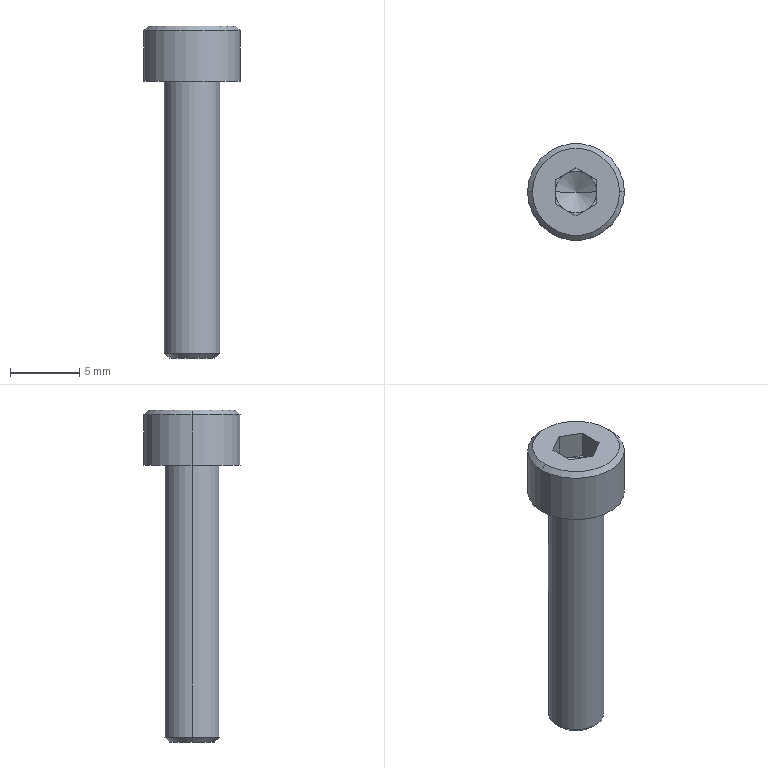Part | SolidWorks | features BaseBody 1 | 1 solid | 25 faces | box 7 x 7 x 24 mm | volume 385.61 mm3 | plane 15 | cone 6 | cylinder 4 | commonest cylinder face diameters 4 x2 7 x2
STEP:
#1=CARTESIAN_POINT('',(2.,0.,-19.65));
#2=VERTEX_POINT('',#1);
#3=CARTESIAN_POINT('',(-2.,0.,-19.65));
#4=VERTEX_POINT('',#3);
#5=CARTESIAN_POINT('',(0.,0.,-19.65));
#6=DIRECTION('',(0.,0.,1.));
#7=DIRECTION('',(1.,0.,0.));
#8=AXIS2_PLACEMENT_3D('',#5,#6,#7);
#9=CIRCLE('',#8,2.);
#10=EDGE_CURVE('',#2,#4,#9,.T.);
#11=ORIENTED_EDGE('',*,*,#10,.T.);
#12=CARTESIAN_POINT('',(-2.,0.,0.));
#13=VERTEX_POINT('',#12);
#14=CARTESIAN_POINT('',(-2.,0.,-20.));
#15=DIRECTION('',(0.,0.,1.));
#16=VECTOR('',#15,1000.);
#17=LINE('',#14,#16);
#18=EDGE_CURVE('',#4,#13,#17,.T.);
#19=ORIENTED_EDGE('',*,*,#18,.T.);
#20=CARTESIAN_POINT('',(2.,0.,0.));
#21=VERTEX_POINT('',#20);
#22=CARTESIAN_POINT('',(0.,0.,0.));
#23=DIRECTION('',(0.,0.,-1.));
#24=DIRECTION('',(1.,0.,0.));
#25=AXIS2_PLACEMENT_3D('',#22,#23,#24);
#26=CIRCLE('',#25,2.);
#27=EDGE_CURVE('',#13,#21,#26,.T.);
#28=ORIENTED_EDGE('',*,*,#27,.T.);
#29=CARTESIAN_POINT('',(2.,0.,-20.));
#30=DIRECTION('',(0.,0.,1.));
#31=VECTOR('',#30,1000.);
#32=LINE('',#29,#31);
#33=EDGE_CURVE('',#2,#21,#32,.T.);
#34=ORIENTED_EDGE('',*,*,#33,.F.);
#35=EDGE_LOOP('',(#11,#19,#28,#34));
#36=FACE_OUTER_BOUND('',#35,.T.);
#37=CARTESIAN_POINT('',(0.,0.,-20.));
#38=DIRECTION('',(0.,0.,1.));
#39=DIRECTION('',(1.,0.,0.));
#40=AXIS2_PLACEMENT_3D('',#37,#38,#39);
#41=CYLINDRICAL_SURFACE('',#40,2.);
#42=ADVANCED_FACE('',(#36),#41,.T.);
#43=CARTESIAN_POINT('',(1.65,0.,-20.));
#44=VERTEX_POINT('',#43);
#45=CARTESIAN_POINT('',(-1.65,0.,-20.));
#46=VERTEX_POINT('',#45);
#47=CARTESIAN_POINT('',(0.,0.,-20.));
#48=DIRECTION('',(0.,0.,1.));
#49=DIRECTION('',(1.,0.,0.));
#50=AXIS2_PLACEMENT_3D('',#47,#48,#49);
#51=CIRCLE('',#50,1.65);
#52=EDGE_CURVE('',#44,#46,#51,.T.);
#53=ORIENTED_EDGE('',*,*,#52,.T.);
#54=CARTESIAN_POINT('',(-2.,0.,-19.65));
#55=DIRECTION('',(-0.7071,0.,0.7071));
#56=VECTOR('',#55,1000.);
#57=LINE('',#54,#56);
#58=EDGE_CURVE('',#46,#4,#57,.T.);
#59=ORIENTED_EDGE('',*,*,#58,.T.);
#60=ORIENTED_EDGE('',*,*,#10,.F.);
#61=CARTESIAN_POINT('',(2.,0.,-19.65));
#62=DIRECTION('',(0.7071,0.,0.7071));
#63=VECTOR('',#62,1000.);
#64=LINE('',#61,#63);
#65=EDGE_CURVE('',#44,#2,#64,.T.);
#66=ORIENTED_EDGE('',*,*,#65,.F.);
#67=EDGE_LOOP('',(#53,#59,#60,#66));
#68=FACE_OUTER_BOUND('',#67,.T.);
#69=CARTESIAN_POINT('',(0.,0.,-19.65));
#70=DIRECTION('',(0.,0.,1.));
#71=DIRECTION('',(1.,0.,0.));
#72=AXIS2_PLACEMENT_3D('',#69,#70,#71);
#73=CONICAL_SURFACE('',#72,2.,0.7854);
#74=ADVANCED_FACE('',(#68),#73,.T.);
#75=CARTESIAN_POINT('',(-3.5,0.,0.));
#76=VERTEX_POINT('',#75);
#77=CARTESIAN_POINT('',(3.5,0.,0.));
#78=VERTEX_POINT('',#77);
#79=CARTESIAN_POINT('',(0.,0.,0.));
#80=DIRECTION('',(0.,0.,-1.));
#81=DIRECTION('',(1.,0.,0.));
#82=AXIS2_PLACEMENT_3D('',#79,#80,#81);
#83=CIRCLE('',#82,3.5);
#84=EDGE_CURVE('',#76,#78,#83,.T.);
#85=ORIENTED_EDGE('',*,*,#84,.F.);
#86=CARTESIAN_POINT('',(-3.5,0.,3.65));
#87=VERTEX_POINT('',#86);
#88=CARTESIAN_POINT('',(-3.5,0.,0.));
#89=DIRECTION('',(0.,0.,1.));
#90=VECTOR('',#89,1000.);
#91=LINE('',#88,#90);
#92=EDGE_CURVE('',#76,#87,#91,.T.);
#93=ORIENTED_EDGE('',*,*,#92,.T.);
#94=CARTESIAN_POINT('',(3.5,0.,3.65));
#95=VERTEX_POINT('',#94);
#96=CARTESIAN_POINT('',(0.,0.,3.65));
#97=DIRECTION('',(0.,0.,-1.));
#98=DIRECTION('',(1.,0.,0.));
#99=AXIS2_PLACEMENT_3D('',#96,#97,#98);
#100=CIRCLE('',#99,3.5);
#101=EDGE_CURVE('',#87,#95,#100,.T.);
#102=ORIENTED_EDGE('',*,*,#101,.T.);
#103=CARTESIAN_POINT('',(3.5,0.,0.));
#104=DIRECTION('',(0.,0.,1.));
#105=VECTOR('',#104,1000.);
#106=LINE('',#103,#105);
#107=EDGE_CURVE('',#78,#95,#106,.T.);
#108=ORIENTED_EDGE('',*,*,#107,.F.);
#109=EDGE_LOOP('',(#85,#93,#102,#108));
#110=FACE_OUTER_BOUND('',#109,.T.);
#111=CARTESIAN_POINT('',(0.,0.,0.));
#112=DIRECTION('',(0.,0.,1.));
#113=DIRECTION('',(1.,0.,0.));
#114=AXIS2_PLACEMENT_3D('',#111,#112,#113);
#115=CYLINDRICAL_SURFACE('',#114,3.5);
#116=ADVANCED_FACE('',(#110),#115,.T.);
#117=CARTESIAN_POINT('',(-3.15,0.,4.));
#118=VERTEX_POINT('',#117);
#119=CARTESIAN_POINT('',(3.15,0.,4.));
#120=VERTEX_POINT('',#119);
#121=CARTESIAN_POINT('',(0.,0.,4.));
#122=DIRECTION('',(0.,0.,-1.));
#123=DIRECTION('',(-1.,0.,0.));
#124=AXIS2_PLACEMENT_3D('',#121,#122,#123);
#125=CIRCLE('',#124,3.15);
#126=EDGE_CURVE('',#118,#120,#125,.T.);
#127=ORIENTED_EDGE('',*,*,#126,.T.);
#128=CARTESIAN_POINT('',(3.5,0.,3.65));
#129=DIRECTION('',(0.7071,0.,-0.7071));
#130=VECTOR('',#129,1000.);
#131=LINE('',#128,#130);
#132=EDGE_CURVE('',#120,#95,#131,.T.);
#133=ORIENTED_EDGE('',*,*,#132,.T.);
#134=ORIENTED_EDGE('',*,*,#101,.F.);
#135=CARTESIAN_POINT('',(-3.5,0.,3.65));
#136=DIRECTION('',(-0.7071,0.,-0.7071));
#137=VECTOR('',#136,1000.);
#138=LINE('',#135,#137);
#139=EDGE_CURVE('',#118,#87,#138,.T.);
#140=ORIENTED_EDGE('',*,*,#139,.F.);
#141=EDGE_LOOP('',(#127,#133,#134,#140));
#142=FACE_OUTER_BOUND('',#141,.T.);
#143=CARTESIAN_POINT('',(0.,0.,3.65));
#144=DIRECTION('',(0.,0.,-1.));
#145=DIRECTION('',(-1.,0.,0.));
#146=AXIS2_PLACEMENT_3D('',#143,#144,#145);
#147=CONICAL_SURFACE('',#146,3.5,0.7854);
#148=ADVANCED_FACE('',(#142),#147,.T.);
#149=CARTESIAN_POINT('',(0.,0.,1.134));
#150=VERTEX_POINT('',#149);
#151=CARTESIAN_POINT('',(1.5,0.,2.));
#152=VERTEX_POINT('',#151);
#153=CARTESIAN_POINT('',(1.5,0.,2.));
#154=DIRECTION('',(0.866,0.,0.5));
#155=VECTOR('',#154,1000.);
#156=LINE('',#153,#155);
#157=EDGE_CURVE('',#150,#152,#156,.T.);
#158=ORIENTED_EDGE('',*,*,#157,.F.);
#159=CARTESIAN_POINT('',(-1.5,0.,2.));
#160=VERTEX_POINT('',#159);
#161=CARTESIAN_POINT('',(-1.5,0.,2.));
#162=DIRECTION('',(-0.866,0.,0.5));
#163=VECTOR('',#162,1000.);
#164=LINE('',#161,#163);
#165=EDGE_CURVE('',#150,#160,#164,.T.);
#166=ORIENTED_EDGE('',*,*,#165,.T.);
#167=CARTESIAN_POINT('',(-0.75,-1.299,2.));
#168=VERTEX_POINT('',#167);
#169=CARTESIAN_POINT('',(0.,0.,2.));
#170=DIRECTION('',(0.,0.,-1.));
#171=DIRECTION('',(1.,0.,0.));
#172=AXIS2_PLACEMENT_3D('',#169,#170,#171);
#173=CIRCLE('',#172,1.5);
#174=EDGE_CURVE('',#168,#160,#173,.T.);
#175=ORIENTED_EDGE('',*,*,#174,.F.);
#176=CARTESIAN_POINT('',(0.75,-1.299,2.));
#177=VERTEX_POINT('',#176);
#178=CARTESIAN_POINT('',(0.,0.,2.));
#179=DIRECTION('',(0.,0.,-1.));
#180=DIRECTION('',(1.,0.,0.));
#181=AXIS2_PLACEMENT_3D('',#178,#179,#180);
#182=CIRCLE('',#181,1.5);
#183=EDGE_CURVE('',#177,#168,#182,.T.);
#184=ORIENTED_EDGE('',*,*,#183,.F.);
#185=CARTESIAN_POINT('',(0.,0.,2.));
#186=DIRECTION('',(0.,0.,-1.));
#187=DIRECTION('',(1.,0.,0.));
#188=AXIS2_PLACEMENT_3D('',#185,#186,#187);
#189=CIRCLE('',#188,1.5);
#190=EDGE_CURVE('',#152,#177,#189,.T.);
#191=ORIENTED_EDGE('',*,*,#190,.F.);
#192=EDGE_LOOP('',(#158,#166,#175,#184,#191));
#193=FACE_OUTER_BOUND('',#192,.T.);
#194=CARTESIAN_POINT('',(0.,0.,2.));
#195=DIRECTION('',(0.,0.,1.));
#196=DIRECTION('',(1.,0.,0.));
#197=AXIS2_PLACEMENT_3D('',#194,#195,#196);
#198=CONICAL_SURFACE('',#197,1.5,1.047);
#199=ADVANCED_FACE('',(#193),#198,.F.);
#200=ORIENTED_EDGE('',*,*,#18,.F.);
#201=CARTESIAN_POINT('',(0.,0.,-19.65));
#202=DIRECTION('',(0.,0.,1.));
#203=DIRECTION('',(1.,0.,0.));
#204=AXIS2_PLACEMENT_3D('',#201,#202,#203);
#205=CIRCLE('',#204,2.);
#206=EDGE_CURVE('',#4,#2,#205,.T.);
#207=ORIENTED_EDGE('',*,*,#206,.T.);
#208=ORIENTED_EDGE('',*,*,#33,.T.);
#209=CARTESIAN_POINT('',(0.,0.,0.));
#210=DIRECTION('',(0.,0.,-1.));
#211=DIRECTION('',(1.,0.,0.));
#212=AXIS2_PLACEMENT_3D('',#209,#210,#211);
#213=CIRCLE('',#212,2.);
#214=EDGE_CURVE('',#21,#13,#213,.T.);
#215=ORIENTED_EDGE('',*,*,#214,.T.);
#216=EDGE_LOOP('',(#200,#207,#208,#215));
#217=FACE_OUTER_BOUND('',#216,.T.);
#218=CARTESIAN_POINT('',(0.,0.,-20.));
#219=DIRECTION('',(0.,0.,1.));
#220=DIRECTION('',(1.,0.,0.));
#221=AXIS2_PLACEMENT_3D('',#218,#219,#220);
#222=CYLINDRICAL_SURFACE('',#221,2.);
#223=ADVANCED_FACE('',(#217),#222,.T.);
#224=CARTESIAN_POINT('',(0.,0.,0.));
#225=DIRECTION('',(0.,0.,-1.));
#226=DIRECTION('',(1.,0.,0.));
#227=AXIS2_PLACEMENT_3D('',#224,#225,#226);
#228=CIRCLE('',#227,3.5);
#229=EDGE_CURVE('',#78,#76,#228,.T.);
#230=ORIENTED_EDGE('',*,*,#229,.T.);
#231=ORIENTED_EDGE('',*,*,#84,.T.);
#232=EDGE_LOOP('',(#230,#231));
#233=FACE_OUTER_BOUND('',#232,.T.);
#234=ORIENTED_EDGE('',*,*,#214,.F.);
#235=ORIENTED_EDGE('',*,*,#27,.F.);
#236=EDGE_LOOP('',(#234,#235));
#237=FACE_BOUND('',#236,.T.);
#238=CARTESIAN_POINT('',(3.5,0.,0.));
#239=DIRECTION('',(0.,0.,-1.));
#240=DIRECTION('',(-1.,0.,0.));
#241=AXIS2_PLACEMENT_3D('',#238,#239,#240);
#242=PLANE('',#241);
#243=ADVANCED_FACE('',(#233,#237),#242,.T.);
#244=ORIENTED_EDGE('',*,*,#58,.F.);
#245=CARTESIAN_POINT('',(0.,0.,-20.));
#246=DIRECTION('',(0.,0.,1.));
#247=DIRECTION('',(1.,0.,0.));
#248=AXIS2_PLACEMENT_3D('',#245,#246,#247);
#249=CIRCLE('',#248,1.65);
#250=EDGE_CURVE('',#46,#44,#249,.T.);
#251=ORIENTED_EDGE('',*,*,#250,.T.);
#252=ORIENTED_EDGE('',*,*,#65,.T.);
#253=ORIENTED_EDGE('',*,*,#206,.F.);
#254=EDGE_LOOP('',(#244,#251,#252,#253));
#255=FACE_OUTER_BOUND('',#254,.T.);
#256=CARTESIAN_POINT('',(0.,0.,-19.65));
#257=DIRECTION('',(0.,0.,1.));
#258=DIRECTION('',(1.,0.,0.));
#259=AXIS2_PLACEMENT_3D('',#256,#257,#258);
#260=CONICAL_SURFACE('',#259,2.,0.7854);
#261=ADVANCED_FACE('',(#255),#260,.T.);
#262=ORIENTED_EDGE('',*,*,#92,.F.);
#263=ORIENTED_EDGE('',*,*,#229,.F.);
#264=ORIENTED_EDGE('',*,*,#107,.T.);
#265=CARTESIAN_POINT('',(0.,0.,3.65));
#266=DIRECTION('',(0.,0.,-1.));
#267=DIRECTION('',(1.,0.,0.));
#268=AXIS2_PLACEMENT_3D('',#265,#266,#267);
#269=CIRCLE('',#268,3.5);
#270=EDGE_CURVE('',#95,#87,#269,.T.);
#271=ORIENTED_EDGE('',*,*,#270,.T.);
#272=EDGE_LOOP('',(#262,#263,#264,#271));
#273=FACE_OUTER_BOUND('',#272,.T.);
#274=CARTESIAN_POINT('',(0.,0.,0.));
#275=DIRECTION('',(0.,0.,1.));
#276=DIRECTION('',(1.,0.,0.));
#277=AXIS2_PLACEMENT_3D('',#274,#275,#276);
#278=CYLINDRICAL_SURFACE('',#277,3.5);
#279=ADVANCED_FACE('',(#273),#278,.T.);
#280=ORIENTED_EDGE('',*,*,#52,.F.);
#281=ORIENTED_EDGE('',*,*,#250,.F.);
#282=EDGE_LOOP('',(#280,#281));
#283=FACE_OUTER_BOUND('',#282,.T.);
#284=CARTESIAN_POINT('',(0.,0.,-20.));
#285=DIRECTION('',(0.,0.,-1.));
#286=DIRECTION('',(-1.,0.,0.));
#287=AXIS2_PLACEMENT_3D('',#284,#285,#286);
#288=PLANE('',#287);
#289=ADVANCED_FACE('',(#283),#288,.T.);
#290=ORIENTED_EDGE('',*,*,#132,.F.);
#291=CARTESIAN_POINT('',(0.,0.,4.));
#292=DIRECTION('',(0.,0.,-1.));
#293=DIRECTION('',(-1.,0.,0.));
#294=AXIS2_PLACEMENT_3D('',#291,#292,#293);
#295=CIRCLE('',#294,3.15);
#296=EDGE_CURVE('',#120,#118,#295,.T.);
#297=ORIENTED_EDGE('',*,*,#296,.T.);
#298=ORIENTED_EDGE('',*,*,#139,.T.);
#299=ORIENTED_EDGE('',*,*,#270,.F.);
#300=EDGE_LOOP('',(#290,#297,#298,#299));
#301=FACE_OUTER_BOUND('',#300,.T.);
#302=CARTESIAN_POINT('',(0.,0.,3.65));
#303=DIRECTION('',(0.,0.,-1.));
#304=DIRECTION('',(-1.,0.,0.));
#305=AXIS2_PLACEMENT_3D('',#302,#303,#304);
#306=CONICAL_SURFACE('',#305,3.5,0.7854);
#307=ADVANCED_FACE('',(#301),#306,.T.);
#308=CARTESIAN_POINT('',(0.,1.732,4.));
#309=VERTEX_POINT('',#308);
#310=CARTESIAN_POINT('',(1.5,0.866,4.));
#311=VERTEX_POINT('',#310);
#312=CARTESIAN_POINT('',(1.5,0.866,4.));
#313=DIRECTION('',(0.866,-0.5,0.));
#314=VECTOR('',#313,1000.);
#315=LINE('',#312,#314);
#316=EDGE_CURVE('',#309,#311,#315,.T.);
#317=ORIENTED_EDGE('',*,*,#316,.T.);
#318=CARTESIAN_POINT('',(1.5,-0.866,4.));
#319=VERTEX_POINT('',#318);
#320=CARTESIAN_POINT('',(1.5,0.,4.));
#321=DIRECTION('',(0.,-1.,0.));
#322=VECTOR('',#321,1000.);
#323=LINE('',#320,#322);
#324=EDGE_CURVE('',#311,#319,#323,.T.);
#325=ORIENTED_EDGE('',*,*,#324,.T.);
#326=CARTESIAN_POINT('',(0.,-1.732,4.));
#327=VERTEX_POINT('',#326);
#328=CARTESIAN_POINT('',(0.,-1.732,4.));
#329=DIRECTION('',(-0.866,-0.5,0.));
#330=VECTOR('',#329,1000.);
#331=LINE('',#328,#330);
#332=EDGE_CURVE('',#319,#327,#331,.T.);
#333=ORIENTED_EDGE('',*,*,#332,.T.);
#334=CARTESIAN_POINT('',(-1.5,-0.866,4.));
#335=VERTEX_POINT('',#334);
#336=CARTESIAN_POINT('',(-1.5,-0.866,4.));
#337=DIRECTION('',(-0.866,0.5,0.));
#338=VECTOR('',#337,1000.);
#339=LINE('',#336,#338);
#340=EDGE_CURVE('',#327,#335,#339,.T.);
#341=ORIENTED_EDGE('',*,*,#340,.T.);
#342=CARTESIAN_POINT('',(-1.5,0.866,4.));
#343=VERTEX_POINT('',#342);
#344=CARTESIAN_POINT('',(-1.5,0.866,4.));
#345=DIRECTION('',(0.,1.,0.));
#346=VECTOR('',#345,1000.);
#347=LINE('',#344,#346);
#348=EDGE_CURVE('',#335,#343,#347,.T.);
#349=ORIENTED_EDGE('',*,*,#348,.T.);
#350=CARTESIAN_POINT('',(0.,1.732,4.));
#351=DIRECTION('',(0.866,0.5,0.));
#352=VECTOR('',#351,1000.);
#353=LINE('',#350,#352);
#354=EDGE_CURVE('',#343,#309,#353,.T.);
#355=ORIENTED_EDGE('',*,*,#354,.T.);
#356=EDGE_LOOP('',(#317,#325,#333,#341,#349,#355));
#357=FACE_BOUND('',#356,.T.);
#358=ORIENTED_EDGE('',*,*,#126,.F.);
#359=ORIENTED_EDGE('',*,*,#296,.F.);
#360=EDGE_LOOP('',(#358,#359));
#361=FACE_OUTER_BOUND('',#360,.T.);
#362=CARTESIAN_POINT('',(0.,0.,4.));
#363=DIRECTION('',(0.,0.,1.));
#364=DIRECTION('',(1.,0.,0.));
#365=AXIS2_PLACEMENT_3D('',#362,#363,#364);
#366=PLANE('',#365);
#367=ADVANCED_FACE('',(#357,#361),#366,.T.);
#368=CARTESIAN_POINT('',(1.5,0.866,2.));
#369=VERTEX_POINT('',#368);
#370=CARTESIAN_POINT('',(1.5,0.866,2.));
#371=DIRECTION('',(0.,0.,1.));
#372=VECTOR('',#371,1000.);
#373=LINE('',#370,#372);
#374=EDGE_CURVE('',#369,#311,#373,.T.);
#375=ORIENTED_EDGE('',*,*,#374,.F.);
#376=CARTESIAN_POINT('',(1.5,-0.866,2.));
#377=DIRECTION('',(0.,1.,0.));
#378=VECTOR('',#377,1000.);
#379=LINE('',#376,#378);
#380=EDGE_CURVE('',#152,#369,#379,.T.);
#381=ORIENTED_EDGE('',*,*,#380,.F.);
#382=CARTESIAN_POINT('',(1.5,-0.866,2.));
#383=VERTEX_POINT('',#382);
#384=CARTESIAN_POINT('',(1.5,-0.866,2.));
#385=DIRECTION('',(0.,1.,0.));
#386=VECTOR('',#385,1000.);
#387=LINE('',#384,#386);
#388=EDGE_CURVE('',#383,#152,#387,.T.);
#389=ORIENTED_EDGE('',*,*,#388,.F.);
#390=CARTESIAN_POINT('',(1.5,-0.866,2.));
#391=DIRECTION('',(0.,0.,-1.));
#392=VECTOR('',#391,1000.);
#393=LINE('',#390,#392);
#394=EDGE_CURVE('',#319,#383,#393,.T.);
#395=ORIENTED_EDGE('',*,*,#394,.F.);
#396=ORIENTED_EDGE('',*,*,#324,.F.);
#397=EDGE_LOOP('',(#375,#381,#389,#395,#396));
#398=FACE_OUTER_BOUND('',#397,.T.);
#399=CARTESIAN_POINT('',(1.5,-0.866,2.));
#400=DIRECTION('',(1.,0.,0.));
#401=DIRECTION('',(0.,1.,0.));
#402=AXIS2_PLACEMENT_3D('',#399,#400,#401);
#403=PLANE('',#402);
#404=ADVANCED_FACE('',(#398),#403,.F.);
#405=CARTESIAN_POINT('',(0.,1.732,2.));
#406=VERTEX_POINT('',#405);
#407=CARTESIAN_POINT('',(0.,1.732,2.));
#408=DIRECTION('',(0.,0.,1.));
#409=VECTOR('',#408,1000.);
#410=LINE('',#407,#409);
#411=EDGE_CURVE('',#406,#309,#410,.T.);
#412=ORIENTED_EDGE('',*,*,#411,.F.);
#413=CARTESIAN_POINT('',(0.75,1.299,2.));
#414=VERTEX_POINT('',#413);
#415=CARTESIAN_POINT('',(1.5,0.866,2.));
#416=DIRECTION('',(-0.866,0.5,0.));
#417=VECTOR('',#416,1000.);
#418=LINE('',#415,#417);
#419=EDGE_CURVE('',#414,#406,#418,.T.);
#420=ORIENTED_EDGE('',*,*,#419,.F.);
#421=CARTESIAN_POINT('',(1.5,0.866,2.));
#422=DIRECTION('',(-0.866,0.5,0.));
#423=VECTOR('',#422,1000.);
#424=LINE('',#421,#423);
#425=EDGE_CURVE('',#369,#414,#424,.T.);
#426=ORIENTED_EDGE('',*,*,#425,.F.);
#427=ORIENTED_EDGE('',*,*,#374,.T.);
#428=ORIENTED_EDGE('',*,*,#316,.F.);
#429=EDGE_LOOP('',(#412,#420,#426,#427,#428));
#430=FACE_OUTER_BOUND('',#429,.T.);
#431=CARTESIAN_POINT('',(1.5,0.866,2.));
#432=DIRECTION('',(0.5,0.866,0.));
#433=DIRECTION('',(-0.866,0.5,0.));
#434=AXIS2_PLACEMENT_3D('',#431,#432,#433);
#435=PLANE('',#434);
#436=ADVANCED_FACE('',(#430),#435,.F.);
#437=CARTESIAN_POINT('',(0.,0.,2.));
#438=DIRECTION('',(0.,0.,-1.));
#439=DIRECTION('',(1.,0.,0.));
#440=AXIS2_PLACEMENT_3D('',#437,#438,#439);
#441=CIRCLE('',#440,1.5);
#442=EDGE_CURVE('',#414,#152,#441,.T.);
#443=ORIENTED_EDGE('',*,*,#442,.T.);
#444=ORIENTED_EDGE('',*,*,#380,.T.);
#445=ORIENTED_EDGE('',*,*,#425,.T.);
#446=EDGE_LOOP('',(#443,#444,#445));
#447=FACE_OUTER_BOUND('',#446,.T.);
#448=CARTESIAN_POINT('',(0.,0.,2.));
#449=DIRECTION('',(0.,0.,1.));
#450=DIRECTION('',(1.,0.,0.));
#451=AXIS2_PLACEMENT_3D('',#448,#449,#450);
#452=PLANE('',#451);
#453=ADVANCED_FACE('',(#447),#452,.T.);
#454=ORIENTED_EDGE('',*,*,#190,.T.);
#455=CARTESIAN_POINT('',(0.75,-1.299,2.));
#456=DIRECTION('',(0.866,0.5,0.));
#457=VECTOR('',#456,1000.);
#458=LINE('',#455,#457);
#459=EDGE_CURVE('',#177,#383,#458,.T.);
#460=ORIENTED_EDGE('',*,*,#459,.T.);
#461=ORIENTED_EDGE('',*,*,#388,.T.);
#462=EDGE_LOOP('',(#454,#460,#461));
#463=FACE_OUTER_BOUND('',#462,.T.);
#464=CARTESIAN_POINT('',(0.,0.,2.));
#465=DIRECTION('',(0.,0.,1.));
#466=DIRECTION('',(1.,0.,0.));
#467=AXIS2_PLACEMENT_3D('',#464,#465,#466);
#468=PLANE('',#467);
#469=ADVANCED_FACE('',(#463),#468,.T.);
#470=ORIENTED_EDGE('',*,*,#394,.T.);
#471=ORIENTED_EDGE('',*,*,#459,.F.);
#472=CARTESIAN_POINT('',(0.,-1.732,2.));
#473=VERTEX_POINT('',#472);
#474=CARTESIAN_POINT('',(0.,-1.732,2.));
#475=DIRECTION('',(0.866,0.5,0.));
#476=VECTOR('',#475,1000.);
#477=LINE('',#474,#476);
#478=EDGE_CURVE('',#473,#177,#477,.T.);
#479=ORIENTED_EDGE('',*,*,#478,.F.);
#480=CARTESIAN_POINT('',(0.,-1.732,2.));
#481=DIRECTION('',(0.,0.,-1.));
#482=VECTOR('',#481,1000.);
#483=LINE('',#480,#482);
#484=EDGE_CURVE('',#327,#473,#483,.T.);
#485=ORIENTED_EDGE('',*,*,#484,.F.);
#486=ORIENTED_EDGE('',*,*,#332,.F.);
#487=EDGE_LOOP('',(#470,#471,#479,#485,#486));
#488=FACE_OUTER_BOUND('',#487,.T.);
#489=CARTESIAN_POINT('',(0.,-1.732,2.));
#490=DIRECTION('',(0.5,-0.866,0.));
#491=DIRECTION('',(0.866,0.5,0.));
#492=AXIS2_PLACEMENT_3D('',#489,#490,#491);
#493=PLANE('',#492);
#494=ADVANCED_FACE('',(#488),#493,.F.);
#495=CARTESIAN_POINT('',(-1.5,0.866,2.));
#496=VERTEX_POINT('',#495);
#497=CARTESIAN_POINT('',(-1.5,0.866,2.));
#498=DIRECTION('',(0.,0.,1.));
#499=VECTOR('',#498,1000.);
#500=LINE('',#497,#499);
#501=EDGE_CURVE('',#496,#343,#500,.T.);
#502=ORIENTED_EDGE('',*,*,#501,.F.);
#503=CARTESIAN_POINT('',(-0.75,1.299,2.));
#504=VERTEX_POINT('',#503);
#505=CARTESIAN_POINT('',(0.,1.732,2.));
#506=DIRECTION('',(-0.866,-0.5,0.));
#507=VECTOR('',#506,1000.);
#508=LINE('',#505,#507);
#509=EDGE_CURVE('',#504,#496,#508,.T.);
#510=ORIENTED_EDGE('',*,*,#509,.F.);
#511=CARTESIAN_POINT('',(0.,1.732,2.));
#512=DIRECTION('',(-0.866,-0.5,0.));
#513=VECTOR('',#512,1000.);
#514=LINE('',#511,#513);
#515=EDGE_CURVE('',#406,#504,#514,.T.);
#516=ORIENTED_EDGE('',*,*,#515,.F.);
#517=ORIENTED_EDGE('',*,*,#411,.T.);
#518=ORIENTED_EDGE('',*,*,#354,.F.);
#519=EDGE_LOOP('',(#502,#510,#516,#517,#518));
#520=FACE_OUTER_BOUND('',#519,.T.);
#521=CARTESIAN_POINT('',(0.,1.732,2.));
#522=DIRECTION('',(-0.5,0.866,0.));
#523=DIRECTION('',(-0.866,-0.5,0.));
#524=AXIS2_PLACEMENT_3D('',#521,#522,#523);
#525=PLANE('',#524);
#526=ADVANCED_FACE('',(#520),#525,.F.);
#527=CARTESIAN_POINT('',(0.,0.,2.));
#528=DIRECTION('',(0.,0.,-1.));
#529=DIRECTION('',(1.,0.,0.));
#530=AXIS2_PLACEMENT_3D('',#527,#528,#529);
#531=CIRCLE('',#530,1.5);
#532=EDGE_CURVE('',#504,#414,#531,.T.);
#533=ORIENTED_EDGE('',*,*,#532,.T.);
#534=ORIENTED_EDGE('',*,*,#419,.T.);
#535=ORIENTED_EDGE('',*,*,#515,.T.);
#536=EDGE_LOOP('',(#533,#534,#535));
#537=FACE_OUTER_BOUND('',#536,.T.);
#538=CARTESIAN_POINT('',(0.,0.,2.));
#539=DIRECTION('',(0.,0.,1.));
#540=DIRECTION('',(1.,0.,0.));
#541=AXIS2_PLACEMENT_3D('',#538,#539,#540);
#542=PLANE('',#541);
#543=ADVANCED_FACE('',(#537),#542,.T.);
#544=ORIENTED_EDGE('',*,*,#165,.F.);
#545=ORIENTED_EDGE('',*,*,#157,.T.);
#546=ORIENTED_EDGE('',*,*,#442,.F.);
#547=ORIENTED_EDGE('',*,*,#532,.F.);
#548=CARTESIAN_POINT('',(0.,0.,2.));
#549=DIRECTION('',(0.,0.,-1.));
#550=DIRECTION('',(1.,0.,0.));
#551=AXIS2_PLACEMENT_3D('',#548,#549,#550);
#552=CIRCLE('',#551,1.5);
#553=EDGE_CURVE('',#160,#504,#552,.T.);
#554=ORIENTED_EDGE('',*,*,#553,.F.);
#555=EDGE_LOOP('',(#544,#545,#546,#547,#554));
#556=FACE_OUTER_BOUND('',#555,.T.);
#557=CARTESIAN_POINT('',(0.,0.,2.));
#558=DIRECTION('',(0.,0.,1.));
#559=DIRECTION('',(1.,0.,0.));
#560=AXIS2_PLACEMENT_3D('',#557,#558,#559);
#561=CONICAL_SURFACE('',#560,1.5,1.047);
#562=ADVANCED_FACE('',(#556),#561,.F.);
#563=ORIENTED_EDGE('',*,*,#183,.T.);
#564=CARTESIAN_POINT('',(-0.75,-1.299,2.));
#565=DIRECTION('',(0.866,-0.5,0.));
#566=VECTOR('',#565,1000.);
#567=LINE('',#564,#566);
#568=EDGE_CURVE('',#168,#473,#567,.T.);
#569=ORIENTED_EDGE('',*,*,#568,.T.);
#570=ORIENTED_EDGE('',*,*,#478,.T.);
#571=EDGE_LOOP('',(#563,#569,#570));
#572=FACE_OUTER_BOUND('',#571,.T.);
#573=CARTESIAN_POINT('',(0.,0.,2.));
#574=DIRECTION('',(0.,0.,1.));
#575=DIRECTION('',(1.,0.,0.));
#576=AXIS2_PLACEMENT_3D('',#573,#574,#575);
#577=PLANE('',#576);
#578=ADVANCED_FACE('',(#572),#577,.T.);
#579=ORIENTED_EDGE('',*,*,#484,.T.);
#580=ORIENTED_EDGE('',*,*,#568,.F.);
#581=CARTESIAN_POINT('',(-1.5,-0.866,2.));
#582=VERTEX_POINT('',#581);
#583=CARTESIAN_POINT('',(-1.5,-0.866,2.));
#584=DIRECTION('',(0.866,-0.5,0.));
#585=VECTOR('',#584,1000.);
#586=LINE('',#583,#585);
#587=EDGE_CURVE('',#582,#168,#586,.T.);
#588=ORIENTED_EDGE('',*,*,#587,.F.);
#589=CARTESIAN_POINT('',(-1.5,-0.866,2.));
#590=DIRECTION('',(0.,0.,-1.));
#591=VECTOR('',#590,1000.);
#592=LINE('',#589,#591);
#593=EDGE_CURVE('',#335,#582,#592,.T.);
#594=ORIENTED_EDGE('',*,*,#593,.F.);
#595=ORIENTED_EDGE('',*,*,#340,.F.);
#596=EDGE_LOOP('',(#579,#580,#588,#594,#595));
#597=FACE_OUTER_BOUND('',#596,.T.);
#598=CARTESIAN_POINT('',(-1.5,-0.866,2.));
#599=DIRECTION('',(-0.5,-0.866,0.));
#600=DIRECTION('',(0.866,-0.5,0.));
#601=AXIS2_PLACEMENT_3D('',#598,#599,#600);
#602=PLANE('',#601);
#603=ADVANCED_FACE('',(#597),#602,.F.);
#604=ORIENTED_EDGE('',*,*,#593,.T.);
#605=CARTESIAN_POINT('',(-1.5,0.866,2.));
#606=DIRECTION('',(0.,-1.,0.));
#607=VECTOR('',#606,1000.);
#608=LINE('',#605,#607);
#609=EDGE_CURVE('',#160,#582,#608,.T.);
#610=ORIENTED_EDGE('',*,*,#609,.F.);
#611=CARTESIAN_POINT('',(-1.5,0.866,2.));
#612=DIRECTION('',(0.,-1.,0.));
#613=VECTOR('',#612,1000.);
#614=LINE('',#611,#613);
#615=EDGE_CURVE('',#496,#160,#614,.T.);
#616=ORIENTED_EDGE('',*,*,#615,.F.);
#617=ORIENTED_EDGE('',*,*,#501,.T.);
#618=ORIENTED_EDGE('',*,*,#348,.F.);
#619=EDGE_LOOP('',(#604,#610,#616,#617,#618));
#620=FACE_OUTER_BOUND('',#619,.T.);
#621=CARTESIAN_POINT('',(-1.5,0.866,2.));
#622=DIRECTION('',(-1.,0.,0.));
#623=DIRECTION('',(0.,-1.,0.));
#624=AXIS2_PLACEMENT_3D('',#621,#622,#623);
#625=PLANE('',#624);
#626=ADVANCED_FACE('',(#620),#625,.F.);
#627=ORIENTED_EDGE('',*,*,#553,.T.);
#628=ORIENTED_EDGE('',*,*,#509,.T.);
#629=ORIENTED_EDGE('',*,*,#615,.T.);
#630=EDGE_LOOP('',(#627,#628,#629));
#631=FACE_OUTER_BOUND('',#630,.T.);
#632=CARTESIAN_POINT('',(0.,0.,2.));
#633=DIRECTION('',(0.,0.,1.));
#634=DIRECTION('',(1.,0.,0.));
#635=AXIS2_PLACEMENT_3D('',#632,#633,#634);
#636=PLANE('',#635);
#637=ADVANCED_FACE('',(#631),#636,.T.);
#638=ORIENTED_EDGE('',*,*,#174,.T.);
#639=ORIENTED_EDGE('',*,*,#609,.T.);
#640=ORIENTED_EDGE('',*,*,#587,.T.);
#641=EDGE_LOOP('',(#638,#639,#640));
#642=FACE_OUTER_BOUND('',#641,.T.);
#643=CARTESIAN_POINT('',(0.,0.,2.));
#644=DIRECTION('',(0.,0.,1.));
#645=DIRECTION('',(1.,0.,0.));
#646=AXIS2_PLACEMENT_3D('',#643,#644,#645);
#647=PLANE('',#646);
#648=ADVANCED_FACE('',(#642),#647,.T.);
#649=CLOSED_SHELL('',(#42,#74,#116,#148,#199,#223,#243,#261,#279,#289,#307,#367,#404,#436,#453,#469,#494,#526,#543,#562,#578,#603,#626,#637,#648));
#650=MANIFOLD_SOLID_BREP('',#649);
#651=CARTESIAN_POINT('',(0.,0.,0.));
#652=DIRECTION('',(0.,0.,1.));
#653=DIRECTION('',(1.,0.,0.));
#654=AXIS2_PLACEMENT_3D('',#651,#652,#653);
#655=(LENGTH_UNIT()NAMED_UNIT(*)SI_UNIT(.MILLI.,.METRE.));
#656=UNCERTAINTY_MEASURE_WITH_UNIT(LENGTH_MEASURE(0.00001),#655,'','');
#657=(NAMED_UNIT(*)PLANE_ANGLE_UNIT()SI_UNIT($,.RADIAN.));
#658=(NAMED_UNIT(*)SI_UNIT($,.STERADIAN.)SOLID_ANGLE_UNIT());
#659=(GEOMETRIC_REPRESENTATION_CONTEXT(3)GLOBAL_UNCERTAINTY_ASSIGNED_CONTEXT((#656))GLOBAL_UNIT_ASSIGNED_CONTEXT((#655,#657,#658))REPRESENTATION_CONTEXT('',''));
#660=ADVANCED_BREP_SHAPE_REPRESENTATION('',(#650,#654),#659);